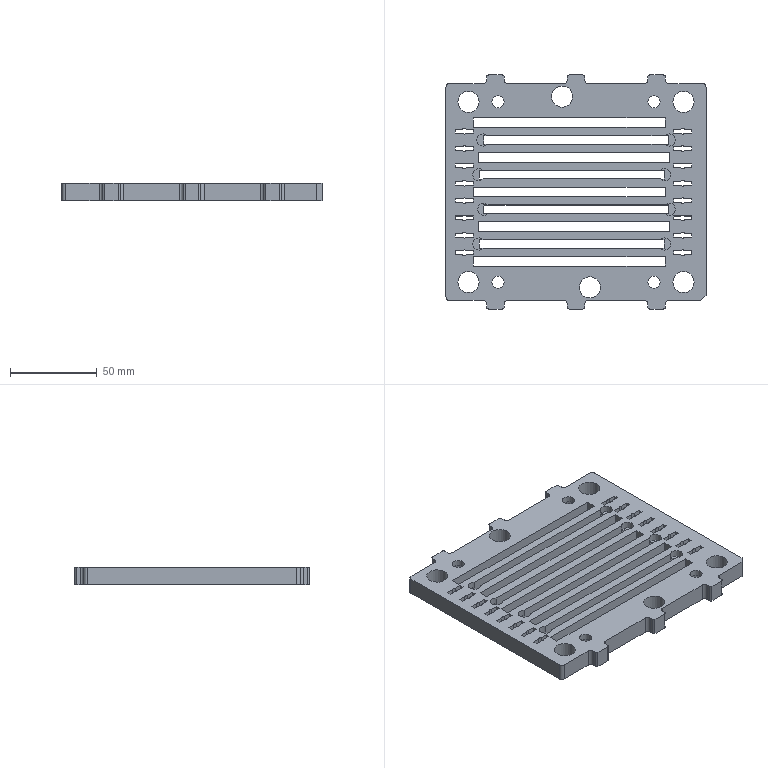Part | STEP file | 1 solid | 256 faces | box 150 x 135 x 10 mm | volume 124052 mm3 | plane 175 | cylinder 81 | commonest cylinder face diameters 3.2 x32 4 x15 2 x12 7 x12 12.2 x6 11 x4